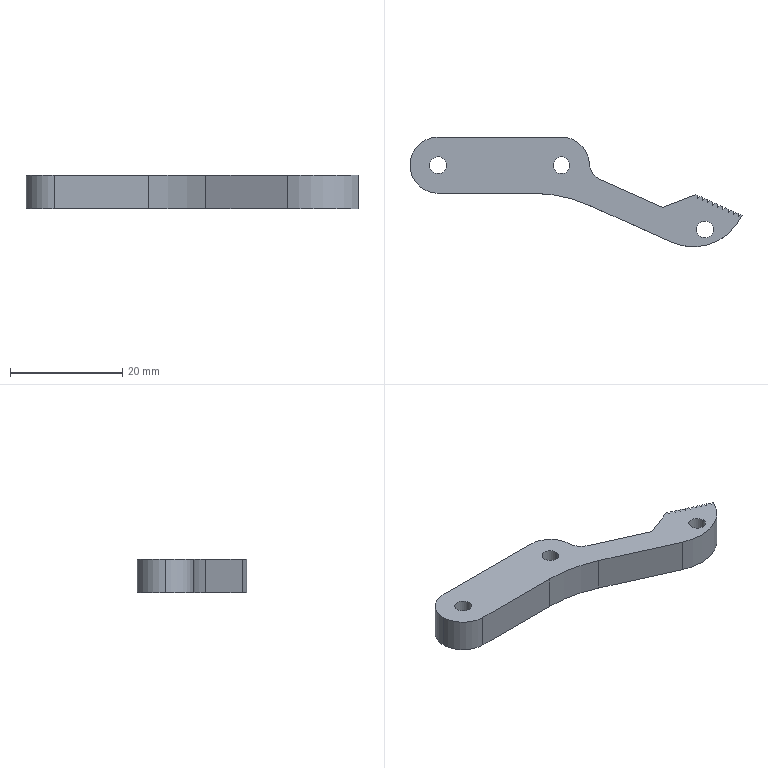Part | STEP file | Long rod_1 | 1 solid | 47 faces | box 59.158 x 19.551 x 6 mm | volume 2724 mm3 | plane 35 | cylinder 12 | commonest cylinder face diameters 3 x6 10 x3 6 x1 19 x1 50 x1